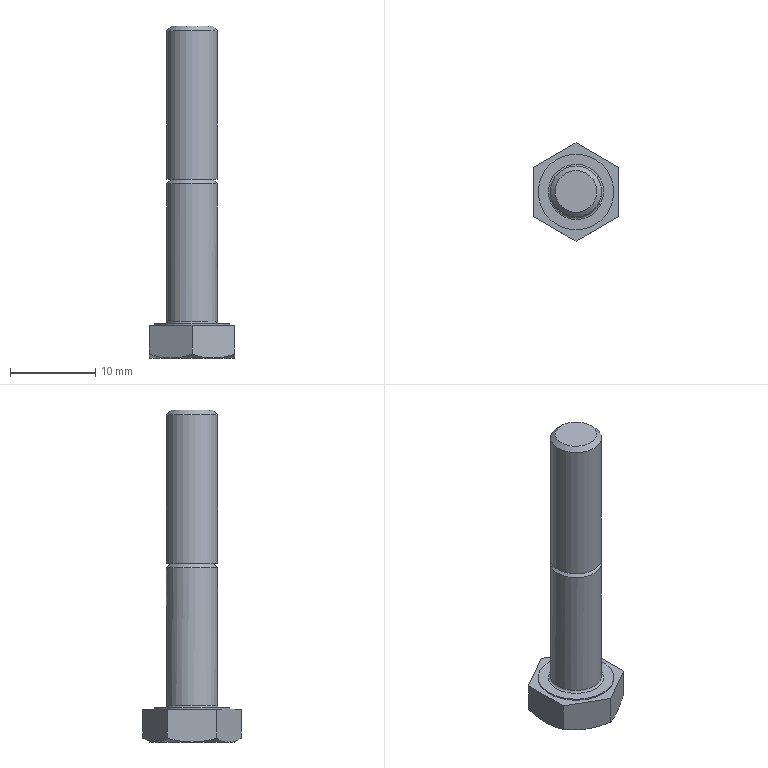Part | STEP file | 1_27 | 1 solid | 23 faces | box 10 x 11.547 x 39 mm | volume 1326 mm3 | plane 11 | cone 8 | cylinder 3 | torus 1 | commonest cylinder face diameters 6 x2 8.88 x1